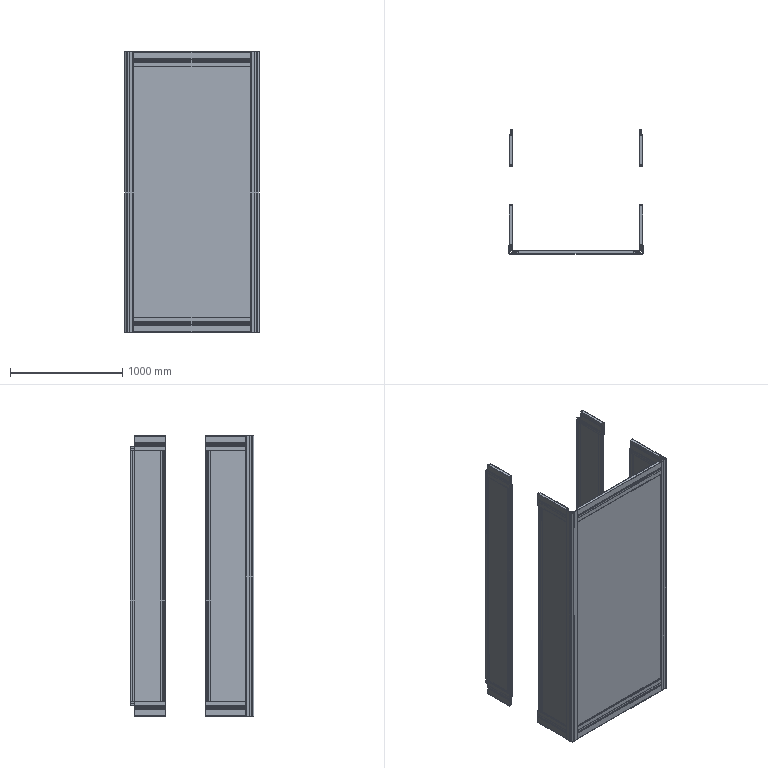Part | SolidWorks | features ReferencePattern 2, MirrorCompFeat 1 | 41 solids | 1657 faces | box 1199 x 1107 x 2502 mm | volume 68599829 mm3 | plane 1222 | cylinder 435 | commonest cylinder face diameters 1.1 x120 3.6 x100 5.8 x100 0.4 x70 10 x32 26 x6